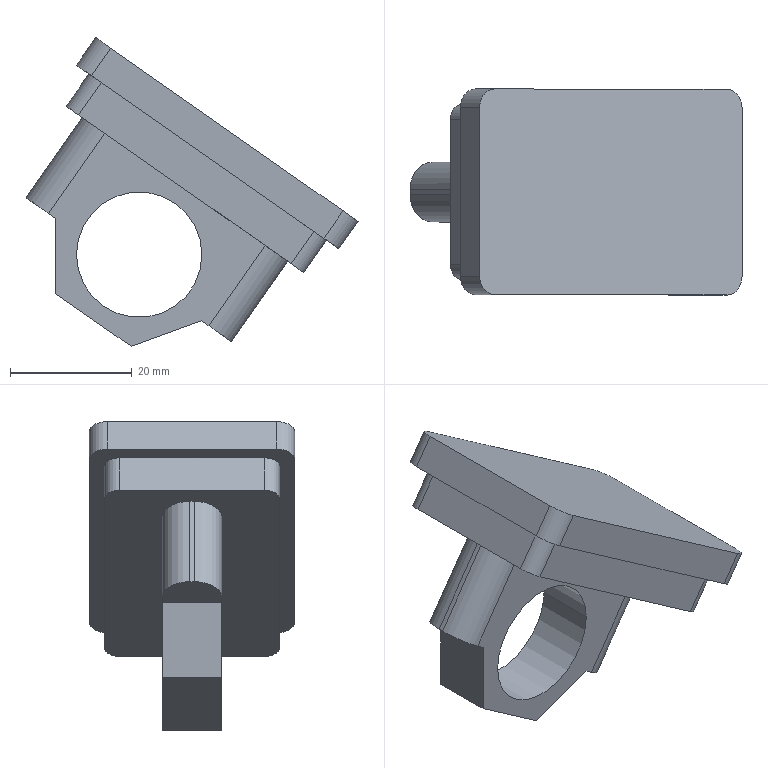Part | SolidWorks | features BaseBody 1 | 1 solid | 34 faces | box 54.536 x 33.8 x 50.697 mm | volume 23757 mm3 | plane 20 | cylinder 14 | commonest cylinder face diameters 5 x4 6 x4 9 x4 20.6 x2
STEP:
#1=CARTESIAN_POINT('',(-249.071,127.55,1106.454));
#2=VERTEX_POINT('',#1);
#3=CARTESIAN_POINT('',(-228.471,127.55,1106.454));
#4=VERTEX_POINT('',#3);
#5=CARTESIAN_POINT('',(-238.771,127.55,1106.454));
#6=DIRECTION('',(0.,-1.,0.));
#7=DIRECTION('',(-1.,0.,0.));
#8=AXIS2_PLACEMENT_3D('',#5,#6,#7);
#9=CIRCLE('',#8,10.3);
#10=EDGE_CURVE('',#2,#4,#9,.T.);
#11=ORIENTED_EDGE('',*,*,#10,.F.);
#12=CARTESIAN_POINT('',(-249.071,117.75,1106.454));
#13=VERTEX_POINT('',#12);
#14=CARTESIAN_POINT('',(-249.071,150.6,1106.454));
#15=DIRECTION('',(0.,-1.,0.));
#16=VECTOR('',#15,1000.);
#17=LINE('',#14,#16);
#18=EDGE_CURVE('',#2,#13,#17,.T.);
#19=ORIENTED_EDGE('',*,*,#18,.T.);
#20=CARTESIAN_POINT('',(-228.471,117.75,1106.454));
#21=VERTEX_POINT('',#20);
#22=CARTESIAN_POINT('',(-238.771,117.75,1106.454));
#23=DIRECTION('',(0.,-1.,0.));
#24=DIRECTION('',(1.,0.,0.));
#25=AXIS2_PLACEMENT_3D('',#22,#23,#24);
#26=CIRCLE('',#25,10.3);
#27=EDGE_CURVE('',#13,#21,#26,.T.);
#28=ORIENTED_EDGE('',*,*,#27,.T.);
#29=CARTESIAN_POINT('',(-228.471,150.6,1106.454));
#30=DIRECTION('',(0.,-1.,0.));
#31=VECTOR('',#30,1000.);
#32=LINE('',#29,#31);
#33=EDGE_CURVE('',#4,#21,#32,.T.);
#34=ORIENTED_EDGE('',*,*,#33,.F.);
#35=EDGE_LOOP('',(#11,#19,#28,#34));
#36=FACE_OUTER_BOUND('',#35,.T.);
#37=CARTESIAN_POINT('',(-238.771,150.6,1106.454));
#38=DIRECTION('',(0.,-1.,0.));
#39=DIRECTION('',(1.,0.,0.));
#40=AXIS2_PLACEMENT_3D('',#37,#38,#39);
#41=CYLINDRICAL_SURFACE('',#40,10.3);
#42=ADVANCED_FACE('',(#36),#41,.F.);
#43=CARTESIAN_POINT('',(-250.753,134.55,1130.836));
#44=VERTEX_POINT('',#43);
#45=CARTESIAN_POINT('',(-248.705,137.05,1129.402));
#46=VERTEX_POINT('',#45);
#47=CARTESIAN_POINT('',(-248.705,134.55,1129.402));
#48=DIRECTION('',(-0.5736,0.,-0.8192));
#49=DIRECTION('',(-0.8192,0.,0.5736));
#50=AXIS2_PLACEMENT_3D('',#47,#48,#49);
#51=CIRCLE('',#50,2.5);
#52=EDGE_CURVE('',#44,#46,#51,.T.);
#53=ORIENTED_EDGE('',*,*,#52,.F.);
#54=CARTESIAN_POINT('',(-247.025,134.55,1136.161));
#55=VERTEX_POINT('',#54);
#56=CARTESIAN_POINT('',(-250.753,134.55,1130.836));
#57=DIRECTION('',(-0.5736,0.,-0.8192));
#58=VECTOR('',#57,1000.);
#59=LINE('',#56,#58);
#60=EDGE_CURVE('',#55,#44,#59,.T.);
#61=ORIENTED_EDGE('',*,*,#60,.F.);
#62=CARTESIAN_POINT('',(-244.977,137.05,1134.727));
#63=VERTEX_POINT('',#62);
#64=CARTESIAN_POINT('',(-244.977,134.55,1134.727));
#65=DIRECTION('',(0.5736,0.,0.8192));
#66=DIRECTION('',(-0.8192,0.,0.5736));
#67=AXIS2_PLACEMENT_3D('',#64,#65,#66);
#68=CIRCLE('',#67,2.5);
#69=EDGE_CURVE('',#63,#55,#68,.T.);
#70=ORIENTED_EDGE('',*,*,#69,.F.);
#71=CARTESIAN_POINT('',(-248.705,137.05,1129.402));
#72=DIRECTION('',(0.5736,0.,0.8192));
#73=VECTOR('',#72,1000.);
#74=LINE('',#71,#73);
#75=EDGE_CURVE('',#46,#63,#74,.T.);
#76=ORIENTED_EDGE('',*,*,#75,.F.);
#77=EDGE_LOOP('',(#53,#61,#70,#76));
#78=FACE_OUTER_BOUND('',#77,.T.);
#79=CARTESIAN_POINT('',(-248.705,134.55,1129.402));
#80=DIRECTION('',(0.5736,0.,0.8192));
#81=DIRECTION('',(-0.8192,0.,0.5736));
#82=AXIS2_PLACEMENT_3D('',#79,#80,#81);
#83=CYLINDRICAL_SURFACE('',#82,2.5);
#84=ADVANCED_FACE('',(#78),#83,.T.);
#85=CARTESIAN_POINT('',(-248.705,108.25,1129.402));
#86=VERTEX_POINT('',#85);
#87=CARTESIAN_POINT('',(-250.753,110.75,1130.836));
#88=VERTEX_POINT('',#87);
#89=CARTESIAN_POINT('',(-248.705,110.75,1129.402));
#90=DIRECTION('',(-0.5736,0.,-0.8192));
#91=DIRECTION('',(-0.8192,0.,0.5736));
#92=AXIS2_PLACEMENT_3D('',#89,#90,#91);
#93=CIRCLE('',#92,2.5);
#94=EDGE_CURVE('',#86,#88,#93,.T.);
#95=ORIENTED_EDGE('',*,*,#94,.F.);
#96=CARTESIAN_POINT('',(-244.977,108.25,1134.727));
#97=VERTEX_POINT('',#96);
#98=CARTESIAN_POINT('',(-248.705,108.25,1129.402));
#99=DIRECTION('',(-0.5736,0.,-0.8192));
#100=VECTOR('',#99,1000.);
#101=LINE('',#98,#100);
#102=EDGE_CURVE('',#97,#86,#101,.T.);
#103=ORIENTED_EDGE('',*,*,#102,.F.);
#104=CARTESIAN_POINT('',(-247.025,110.75,1136.161));
#105=VERTEX_POINT('',#104);
#106=CARTESIAN_POINT('',(-244.977,110.75,1134.727));
#107=DIRECTION('',(0.5736,0.,0.8192));
#108=DIRECTION('',(-0.8192,0.,0.5736));
#109=AXIS2_PLACEMENT_3D('',#106,#107,#108);
#110=CIRCLE('',#109,2.5);
#111=EDGE_CURVE('',#105,#97,#110,.T.);
#112=ORIENTED_EDGE('',*,*,#111,.F.);
#113=CARTESIAN_POINT('',(-250.753,110.75,1130.836));
#114=DIRECTION('',(0.5736,0.,0.8192));
#115=VECTOR('',#114,1000.);
#116=LINE('',#113,#115);
#117=EDGE_CURVE('',#88,#105,#116,.T.);
#118=ORIENTED_EDGE('',*,*,#117,.F.);
#119=EDGE_LOOP('',(#95,#103,#112,#118));
#120=FACE_OUTER_BOUND('',#119,.T.);
#121=CARTESIAN_POINT('',(-248.705,110.75,1129.402));
#122=DIRECTION('',(0.5736,0.,0.8192));
#123=DIRECTION('',(-0.8192,0.,0.5736));
#124=AXIS2_PLACEMENT_3D('',#121,#122,#123);
#125=CYLINDRICAL_SURFACE('',#124,2.5);
#126=ADVANCED_FACE('',(#120),#125,.T.);
#127=CARTESIAN_POINT('',(-211.761,110.75,1103.534));
#128=VERTEX_POINT('',#127);
#129=CARTESIAN_POINT('',(-213.809,108.25,1104.968));
#130=VERTEX_POINT('',#129);
#131=CARTESIAN_POINT('',(-213.809,110.75,1104.968));
#132=DIRECTION('',(-0.5736,0.,-0.8192));
#133=DIRECTION('',(-0.8192,0.,0.5736));
#134=AXIS2_PLACEMENT_3D('',#131,#132,#133);
#135=CIRCLE('',#134,2.5);
#136=EDGE_CURVE('',#128,#130,#135,.T.);
#137=ORIENTED_EDGE('',*,*,#136,.F.);
#138=CARTESIAN_POINT('',(-208.033,110.75,1108.858));
#139=VERTEX_POINT('',#138);
#140=CARTESIAN_POINT('',(-211.761,110.75,1103.534));
#141=DIRECTION('',(-0.5736,0.,-0.8192));
#142=VECTOR('',#141,1000.);
#143=LINE('',#140,#142);
#144=EDGE_CURVE('',#139,#128,#143,.T.);
#145=ORIENTED_EDGE('',*,*,#144,.F.);
#146=CARTESIAN_POINT('',(-210.081,108.25,1110.292));
#147=VERTEX_POINT('',#146);
#148=CARTESIAN_POINT('',(-210.081,110.75,1110.292));
#149=DIRECTION('',(0.5736,0.,0.8192));
#150=DIRECTION('',(-0.8192,0.,0.5736));
#151=AXIS2_PLACEMENT_3D('',#148,#149,#150);
#152=CIRCLE('',#151,2.5);
#153=EDGE_CURVE('',#147,#139,#152,.T.);
#154=ORIENTED_EDGE('',*,*,#153,.F.);
#155=CARTESIAN_POINT('',(-213.809,108.25,1104.968));
#156=DIRECTION('',(0.5736,0.,0.8192));
#157=VECTOR('',#156,1000.);
#158=LINE('',#155,#157);
#159=EDGE_CURVE('',#130,#147,#158,.T.);
#160=ORIENTED_EDGE('',*,*,#159,.F.);
#161=EDGE_LOOP('',(#137,#145,#154,#160));
#162=FACE_OUTER_BOUND('',#161,.T.);
#163=CARTESIAN_POINT('',(-213.809,110.75,1104.968));
#164=DIRECTION('',(0.5736,0.,0.8192));
#165=DIRECTION('',(-0.8192,0.,0.5736));
#166=AXIS2_PLACEMENT_3D('',#163,#164,#165);
#167=CYLINDRICAL_SURFACE('',#166,2.5);
#168=ADVANCED_FACE('',(#162),#167,.T.);
#169=CARTESIAN_POINT('',(-213.809,137.05,1104.968));
#170=VERTEX_POINT('',#169);
#171=CARTESIAN_POINT('',(-211.761,134.55,1103.534));
#172=VERTEX_POINT('',#171);
#173=CARTESIAN_POINT('',(-213.809,134.55,1104.968));
#174=DIRECTION('',(-0.5736,0.,-0.8192));
#175=DIRECTION('',(-0.8192,0.,0.5736));
#176=AXIS2_PLACEMENT_3D('',#173,#174,#175);
#177=CIRCLE('',#176,2.5);
#178=EDGE_CURVE('',#170,#172,#177,.T.);
#179=ORIENTED_EDGE('',*,*,#178,.F.);
#180=CARTESIAN_POINT('',(-210.081,137.05,1110.292));
#181=VERTEX_POINT('',#180);
#182=CARTESIAN_POINT('',(-213.809,137.05,1104.968));
#183=DIRECTION('',(-0.5736,0.,-0.8192));
#184=VECTOR('',#183,1000.);
#185=LINE('',#182,#184);
#186=EDGE_CURVE('',#181,#170,#185,.T.);
#187=ORIENTED_EDGE('',*,*,#186,.F.);
#188=CARTESIAN_POINT('',(-208.033,134.55,1108.858));
#189=VERTEX_POINT('',#188);
#190=CARTESIAN_POINT('',(-210.081,134.55,1110.292));
#191=DIRECTION('',(0.5736,0.,0.8192));
#192=DIRECTION('',(-0.8192,0.,0.5736));
#193=AXIS2_PLACEMENT_3D('',#190,#191,#192);
#194=CIRCLE('',#193,2.5);
#195=EDGE_CURVE('',#189,#181,#194,.T.);
#196=ORIENTED_EDGE('',*,*,#195,.F.);
#197=CARTESIAN_POINT('',(-211.761,134.55,1103.534));
#198=DIRECTION('',(0.5736,0.,0.8192));
#199=VECTOR('',#198,1000.);
#200=LINE('',#197,#199);
#201=EDGE_CURVE('',#172,#189,#200,.T.);
#202=ORIENTED_EDGE('',*,*,#201,.F.);
#203=EDGE_LOOP('',(#179,#187,#196,#202));
#204=FACE_OUTER_BOUND('',#203,.T.);
#205=CARTESIAN_POINT('',(-213.809,134.55,1104.968));
#206=DIRECTION('',(0.5736,0.,0.8192));
#207=DIRECTION('',(-0.8192,0.,0.5736));
#208=AXIS2_PLACEMENT_3D('',#205,#206,#207);
#209=CYLINDRICAL_SURFACE('',#208,2.5);
#210=ADVANCED_FACE('',(#204),#209,.T.);
#211=CARTESIAN_POINT('',(-249.073,136.55,1137.595));
#212=VERTEX_POINT('',#211);
#213=CARTESIAN_POINT('',(-246.615,139.55,1135.874));
#214=VERTEX_POINT('',#213);
#215=CARTESIAN_POINT('',(-246.615,136.55,1135.874));
#216=DIRECTION('',(-0.5736,0.,-0.8192));
#217=DIRECTION('',(-0.8192,0.,0.5736));
#218=AXIS2_PLACEMENT_3D('',#215,#216,#217);
#219=CIRCLE('',#218,3.);
#220=EDGE_CURVE('',#212,#214,#219,.T.);
#221=ORIENTED_EDGE('',*,*,#220,.F.);
#222=CARTESIAN_POINT('',(-245.918,136.55,1142.1));
#223=VERTEX_POINT('',#222);
#224=CARTESIAN_POINT('',(-249.073,136.55,1137.595));
#225=DIRECTION('',(-0.5736,0.,-0.8192));
#226=VECTOR('',#225,1000.);
#227=LINE('',#224,#226);
#228=EDGE_CURVE('',#223,#212,#227,.T.);
#229=ORIENTED_EDGE('',*,*,#228,.F.);
#230=CARTESIAN_POINT('',(-243.461,139.55,1140.379));
#231=VERTEX_POINT('',#230);
#232=CARTESIAN_POINT('',(-243.461,136.55,1140.379));
#233=DIRECTION('',(0.5736,0.,0.8192));
#234=DIRECTION('',(-0.8192,0.,0.5736));
#235=AXIS2_PLACEMENT_3D('',#232,#233,#234);
#236=CIRCLE('',#235,3.);
#237=EDGE_CURVE('',#231,#223,#236,.T.);
#238=ORIENTED_EDGE('',*,*,#237,.F.);
#239=CARTESIAN_POINT('',(-246.615,139.55,1135.874));
#240=DIRECTION('',(0.5736,0.,0.8192));
#241=VECTOR('',#240,1000.);
#242=LINE('',#239,#241);
#243=EDGE_CURVE('',#214,#231,#242,.T.);
#244=ORIENTED_EDGE('',*,*,#243,.F.);
#245=EDGE_LOOP('',(#221,#229,#238,#244));
#246=FACE_OUTER_BOUND('',#245,.T.);
#247=CARTESIAN_POINT('',(-246.615,136.55,1135.874));
#248=DIRECTION('',(0.5736,0.,0.8192));
#249=DIRECTION('',(-0.8192,0.,0.5736));
#250=AXIS2_PLACEMENT_3D('',#247,#248,#249);
#251=CYLINDRICAL_SURFACE('',#250,3.);
#252=ADVANCED_FACE('',(#246),#251,.T.);
#253=CARTESIAN_POINT('',(-208.443,139.55,1109.145));
#254=VERTEX_POINT('',#253);
#255=CARTESIAN_POINT('',(-205.985,136.55,1107.425));
#256=VERTEX_POINT('',#255);
#257=CARTESIAN_POINT('',(-208.443,136.55,1109.145));
#258=DIRECTION('',(-0.5736,0.,-0.8192));
#259=DIRECTION('',(-0.8192,0.,0.5736));
#260=AXIS2_PLACEMENT_3D('',#257,#258,#259);
#261=CIRCLE('',#260,3.);
#262=EDGE_CURVE('',#254,#256,#261,.T.);
#263=ORIENTED_EDGE('',*,*,#262,.F.);
#264=CARTESIAN_POINT('',(-205.288,139.55,1113.651));
#265=VERTEX_POINT('',#264);
#266=CARTESIAN_POINT('',(-208.443,139.55,1109.145));
#267=DIRECTION('',(-0.5736,0.,-0.8192));
#268=VECTOR('',#267,1000.);
#269=LINE('',#266,#268);
#270=EDGE_CURVE('',#265,#254,#269,.T.);
#271=ORIENTED_EDGE('',*,*,#270,.F.);
#272=CARTESIAN_POINT('',(-202.831,136.55,1111.93));
#273=VERTEX_POINT('',#272);
#274=CARTESIAN_POINT('',(-205.288,136.55,1113.651));
#275=DIRECTION('',(0.5736,0.,0.8192));
#276=DIRECTION('',(-0.8192,0.,0.5736));
#277=AXIS2_PLACEMENT_3D('',#274,#275,#276);
#278=CIRCLE('',#277,3.);
#279=EDGE_CURVE('',#273,#265,#278,.T.);
#280=ORIENTED_EDGE('',*,*,#279,.F.);
#281=CARTESIAN_POINT('',(-205.985,136.55,1107.425));
#282=DIRECTION('',(0.5736,0.,0.8192));
#283=VECTOR('',#282,1000.);
#284=LINE('',#281,#283);
#285=EDGE_CURVE('',#256,#273,#284,.T.);
#286=ORIENTED_EDGE('',*,*,#285,.F.);
#287=EDGE_LOOP('',(#263,#271,#280,#286));
#288=FACE_OUTER_BOUND('',#287,.T.);
#289=CARTESIAN_POINT('',(-208.443,136.55,1109.145));
#290=DIRECTION('',(0.5736,0.,0.8192));
#291=DIRECTION('',(-0.8192,0.,0.5736));
#292=AXIS2_PLACEMENT_3D('',#289,#290,#291);
#293=CYLINDRICAL_SURFACE('',#292,3.);
#294=ADVANCED_FACE('',(#288),#293,.T.);
#295=CARTESIAN_POINT('',(-205.985,108.75,1107.425));
#296=VERTEX_POINT('',#295);
#297=CARTESIAN_POINT('',(-208.443,105.75,1109.145));
#298=VERTEX_POINT('',#297);
#299=CARTESIAN_POINT('',(-208.443,108.75,1109.145));
#300=DIRECTION('',(-0.5736,0.,-0.8192));
#301=DIRECTION('',(-0.8192,0.,0.5736));
#302=AXIS2_PLACEMENT_3D('',#299,#300,#301);
#303=CIRCLE('',#302,3.);
#304=EDGE_CURVE('',#296,#298,#303,.T.);
#305=ORIENTED_EDGE('',*,*,#304,.F.);
#306=CARTESIAN_POINT('',(-202.831,108.75,1111.93));
#307=VERTEX_POINT('',#306);
#308=CARTESIAN_POINT('',(-205.985,108.75,1107.425));
#309=DIRECTION('',(-0.5736,0.,-0.8192));
#310=VECTOR('',#309,1000.);
#311=LINE('',#308,#310);
#312=EDGE_CURVE('',#307,#296,#311,.T.);
#313=ORIENTED_EDGE('',*,*,#312,.F.);
#314=CARTESIAN_POINT('',(-205.288,105.75,1113.651));
#315=VERTEX_POINT('',#314);
#316=CARTESIAN_POINT('',(-205.288,108.75,1113.651));
#317=DIRECTION('',(0.5736,0.,0.8192));
#318=DIRECTION('',(-0.8192,0.,0.5736));
#319=AXIS2_PLACEMENT_3D('',#316,#317,#318);
#320=CIRCLE('',#319,3.);
#321=EDGE_CURVE('',#315,#307,#320,.T.);
#322=ORIENTED_EDGE('',*,*,#321,.F.);
#323=CARTESIAN_POINT('',(-208.443,105.75,1109.145));
#324=DIRECTION('',(0.5736,0.,0.8192));
#325=VECTOR('',#324,1000.);
#326=LINE('',#323,#325);
#327=EDGE_CURVE('',#298,#315,#326,.T.);
#328=ORIENTED_EDGE('',*,*,#327,.F.);
#329=EDGE_LOOP('',(#305,#313,#322,#328));
#330=FACE_OUTER_BOUND('',#329,.T.);
#331=CARTESIAN_POINT('',(-208.443,108.75,1109.145));
#332=DIRECTION('',(0.5736,0.,0.8192));
#333=DIRECTION('',(-0.8192,0.,0.5736));
#334=AXIS2_PLACEMENT_3D('',#331,#332,#333);
#335=CYLINDRICAL_SURFACE('',#334,3.);
#336=ADVANCED_FACE('',(#330),#335,.T.);
#337=CARTESIAN_POINT('',(-246.615,105.75,1135.874));
#338=VERTEX_POINT('',#337);
#339=CARTESIAN_POINT('',(-249.073,108.75,1137.595));
#340=VERTEX_POINT('',#339);
#341=CARTESIAN_POINT('',(-246.615,108.75,1135.874));
#342=DIRECTION('',(-0.5736,0.,-0.8192));
#343=DIRECTION('',(-0.8192,0.,0.5736));
#344=AXIS2_PLACEMENT_3D('',#341,#342,#343);
#345=CIRCLE('',#344,3.);
#346=EDGE_CURVE('',#338,#340,#345,.T.);
#347=ORIENTED_EDGE('',*,*,#346,.F.);
#348=CARTESIAN_POINT('',(-243.461,105.75,1140.379));
#349=VERTEX_POINT('',#348);
#350=CARTESIAN_POINT('',(-246.615,105.75,1135.874));
#351=DIRECTION('',(-0.5736,0.,-0.8192));
#352=VECTOR('',#351,1000.);
#353=LINE('',#350,#352);
#354=EDGE_CURVE('',#349,#338,#353,.T.);
#355=ORIENTED_EDGE('',*,*,#354,.F.);
#356=CARTESIAN_POINT('',(-245.918,108.75,1142.1));
#357=VERTEX_POINT('',#356);
#358=CARTESIAN_POINT('',(-243.461,108.75,1140.379));
#359=DIRECTION('',(0.5736,0.,0.8192));
#360=DIRECTION('',(-0.8192,0.,0.5736));
#361=AXIS2_PLACEMENT_3D('',#358,#359,#360);
#362=CIRCLE('',#361,3.);
#363=EDGE_CURVE('',#357,#349,#362,.T.);
#364=ORIENTED_EDGE('',*,*,#363,.F.);
#365=CARTESIAN_POINT('',(-249.073,108.75,1137.595));
#366=DIRECTION('',(0.5736,0.,0.8192));
#367=VECTOR('',#366,1000.);
#368=LINE('',#365,#367);
#369=EDGE_CURVE('',#340,#357,#368,.T.);
#370=ORIENTED_EDGE('',*,*,#369,.F.);
#371=EDGE_LOOP('',(#347,#355,#364,#370));
#372=FACE_OUTER_BOUND('',#371,.T.);
#373=CARTESIAN_POINT('',(-246.615,108.75,1135.874));
#374=DIRECTION('',(0.5736,0.,0.8192));
#375=DIRECTION('',(-0.8192,0.,0.5736));
#376=AXIS2_PLACEMENT_3D('',#373,#374,#375);
#377=CYLINDRICAL_SURFACE('',#376,3.);
#378=ADVANCED_FACE('',(#372),#377,.T.);
#379=CARTESIAN_POINT('',(-252.455,127.55,1112.373));
#380=VERTEX_POINT('',#379);
#381=CARTESIAN_POINT('',(-252.455,117.75,1112.373));
#382=VERTEX_POINT('',#381);
#383=CARTESIAN_POINT('',(-252.455,235.55,1112.373));
#384=DIRECTION('',(0.,-1.,0.));
#385=VECTOR('',#384,1000.);
#386=LINE('',#383,#385);
#387=EDGE_CURVE('',#380,#382,#386,.T.);
#388=ORIENTED_EDGE('',*,*,#387,.T.);
#389=CARTESIAN_POINT('',(-253.68,117.75,1113.231));
#390=VERTEX_POINT('',#389);
#391=CARTESIAN_POINT('',(-240.492,117.75,1103.997));
#392=DIRECTION('',(0.8192,0.,-0.5736));
#393=VECTOR('',#392,1000.);
#394=LINE('',#391,#393);
#395=EDGE_CURVE('',#390,#382,#394,.T.);
#396=ORIENTED_EDGE('',*,*,#395,.F.);
#397=CARTESIAN_POINT('',(-257.366,122.25,1115.812));
#398=VERTEX_POINT('',#397);
#399=CARTESIAN_POINT('',(-253.68,122.25,1113.231));
#400=DIRECTION('',(0.5736,0.,0.8192));
#401=DIRECTION('',(-0.8192,0.,0.5736));
#402=AXIS2_PLACEMENT_3D('',#399,#400,#401);
#403=CIRCLE('',#402,4.5);
#404=EDGE_CURVE('',#398,#390,#403,.T.);
#405=ORIENTED_EDGE('',*,*,#404,.F.);
#406=CARTESIAN_POINT('',(-257.366,123.05,1115.812));
#407=VERTEX_POINT('',#406);
#408=CARTESIAN_POINT('',(-257.366,134.05,1115.812));
#409=DIRECTION('',(0.,1.,0.));
#410=VECTOR('',#409,1000.);
#411=LINE('',#408,#410);
#412=EDGE_CURVE('',#398,#407,#411,.T.);
#413=ORIENTED_EDGE('',*,*,#412,.T.);
#414=CARTESIAN_POINT('',(-253.68,127.55,1113.231));
#415=VERTEX_POINT('',#414);
#416=CARTESIAN_POINT('',(-253.68,123.05,1113.231));
#417=DIRECTION('',(0.5736,0.,0.8192));
#418=DIRECTION('',(-0.8192,0.,0.5736));
#419=AXIS2_PLACEMENT_3D('',#416,#417,#418);
#420=CIRCLE('',#419,4.5);
#421=EDGE_CURVE('',#415,#407,#420,.T.);
#422=ORIENTED_EDGE('',*,*,#421,.F.);
#423=CARTESIAN_POINT('',(439.589,127.55,627.799));
#424=DIRECTION('',(0.8192,0.,-0.5736));
#425=VECTOR('',#424,1000.);
#426=LINE('',#423,#425);
#427=EDGE_CURVE('',#415,#380,#426,.T.);
#428=ORIENTED_EDGE('',*,*,#427,.T.);
#429=EDGE_LOOP('',(#388,#396,#405,#413,#422,#428));
#430=FACE_OUTER_BOUND('',#429,.T.);
#431=CARTESIAN_POINT('',(-252.455,235.55,1112.373));
#432=DIRECTION('',(-0.5736,0.,-0.8192));
#433=DIRECTION('',(-0.8192,0.,0.5736));
#434=AXIS2_PLACEMENT_3D('',#431,#432,#433);
#435=PLANE('',#434);
#436=ADVANCED_FACE('',(#430),#435,.T.);
#437=CARTESIAN_POINT('',(-252.455,127.55,1100.043));
#438=VERTEX_POINT('',#437);
#439=CARTESIAN_POINT('',(-252.455,117.75,1100.043));
#440=VERTEX_POINT('',#439);
#441=CARTESIAN_POINT('',(-252.455,122.65,1100.043));
#442=DIRECTION('',(0.,-1.,0.));
#443=VECTOR('',#442,1000.);
#444=LINE('',#441,#443);
#445=EDGE_CURVE('',#438,#440,#444,.T.);
#446=ORIENTED_EDGE('',*,*,#445,.T.);
#447=CARTESIAN_POINT('',(-252.455,117.75,1122.51));
#448=DIRECTION('',(0.,0.,-1.));
#449=VECTOR('',#448,1000.);
#450=LINE('',#447,#449);
#451=EDGE_CURVE('',#382,#440,#450,.T.);
#452=ORIENTED_EDGE('',*,*,#451,.F.);
#453=ORIENTED_EDGE('',*,*,#387,.F.);
#454=CARTESIAN_POINT('',(-252.455,127.55,-21.38));
#455=DIRECTION('',(0.,0.,-1.));
#456=VECTOR('',#455,1000.);
#457=LINE('',#454,#456);
#458=EDGE_CURVE('',#380,#438,#457,.T.);
#459=ORIENTED_EDGE('',*,*,#458,.T.);
#460=EDGE_LOOP('',(#446,#452,#453,#459));
#461=FACE_OUTER_BOUND('',#460,.T.);
#462=CARTESIAN_POINT('',(-252.455,235.55,1112.373));
#463=DIRECTION('',(-1.,0.,0.));
#464=DIRECTION('',(0.,0.,1.));
#465=AXIS2_PLACEMENT_3D('',#462,#463,#464);
#466=PLANE('',#465);
#467=ADVANCED_FACE('',(#461),#466,.T.);
#468=CARTESIAN_POINT('',(-227.303,117.75,1094.762));
#469=VERTEX_POINT('',#468);
#470=CARTESIAN_POINT('',(-223.617,122.25,1092.181));
#471=VERTEX_POINT('',#470);
#472=CARTESIAN_POINT('',(-227.303,122.25,1094.762));
#473=DIRECTION('',(0.5736,0.,0.8192));
#474=DIRECTION('',(-0.8192,0.,0.5736));
#475=AXIS2_PLACEMENT_3D('',#472,#473,#474);
#476=CIRCLE('',#475,4.5);
#477=EDGE_CURVE('',#469,#471,#476,.T.);
#478=ORIENTED_EDGE('',*,*,#477,.F.);
#479=CARTESIAN_POINT('',(-228.529,117.75,1095.62));
#480=VERTEX_POINT('',#479);
#481=CARTESIAN_POINT('',(-240.492,117.75,1103.997));
#482=DIRECTION('',(0.8192,0.,-0.5736));
#483=VECTOR('',#482,1000.);
#484=LINE('',#481,#483);
#485=EDGE_CURVE('',#480,#469,#484,.T.);
#486=ORIENTED_EDGE('',*,*,#485,.F.);
#487=CARTESIAN_POINT('',(-228.529,127.55,1095.62));
#488=VERTEX_POINT('',#487);
#489=CARTESIAN_POINT('',(-228.529,235.55,1095.62));
#490=DIRECTION('',(0.,-1.,0.));
#491=VECTOR('',#490,1000.);
#492=LINE('',#489,#491);
#493=EDGE_CURVE('',#488,#480,#492,.T.);
#494=ORIENTED_EDGE('',*,*,#493,.F.);
#495=CARTESIAN_POINT('',(-227.303,127.55,1094.762));
#496=VERTEX_POINT('',#495);
#497=CARTESIAN_POINT('',(439.589,127.55,627.799));
#498=DIRECTION('',(0.8192,0.,-0.5736));
#499=VECTOR('',#498,1000.);
#500=LINE('',#497,#499);
#501=EDGE_CURVE('',#488,#496,#500,.T.);
#502=ORIENTED_EDGE('',*,*,#501,.T.);
#503=CARTESIAN_POINT('',(-223.617,123.05,1092.181));
#504=VERTEX_POINT('',#503);
#505=CARTESIAN_POINT('',(-227.303,123.05,1094.762));
#506=DIRECTION('',(0.5736,0.,0.8192));
#507=DIRECTION('',(-0.8192,0.,0.5736));
#508=AXIS2_PLACEMENT_3D('',#505,#506,#507);
#509=CIRCLE('',#508,4.5);
#510=EDGE_CURVE('',#504,#496,#509,.T.);
#511=ORIENTED_EDGE('',*,*,#510,.F.);
#512=CARTESIAN_POINT('',(-223.617,134.05,1092.181));
#513=DIRECTION('',(0.,-1.,0.));
#514=VECTOR('',#513,1000.);
#515=LINE('',#512,#514);
#516=EDGE_CURVE('',#504,#471,#515,.T.);
#517=ORIENTED_EDGE('',*,*,#516,.T.);
#518=EDGE_LOOP('',(#478,#486,#494,#502,#511,#517));
#519=FACE_OUTER_BOUND('',#518,.T.);
#520=CARTESIAN_POINT('',(-216.531,235.55,1087.219));
#521=DIRECTION('',(-0.5736,0.,-0.8192));
#522=DIRECTION('',(-0.8192,0.,0.5736));
#523=AXIS2_PLACEMENT_3D('',#520,#521,#522);
#524=PLANE('',#523);
#525=ADVANCED_FACE('',(#519),#524,.T.);
#526=ORIENTED_EDGE('',*,*,#493,.T.);
#527=CARTESIAN_POINT('',(-240.115,117.75,1091.403));
#528=VERTEX_POINT('',#527);
#529=CARTESIAN_POINT('',(-219.004,117.75,1099.087));
#530=DIRECTION('',(0.9397,0.,0.342));
#531=VECTOR('',#530,1000.);
#532=LINE('',#529,#531);
#533=EDGE_CURVE('',#528,#480,#532,.T.);
#534=ORIENTED_EDGE('',*,*,#533,.F.);
#535=CARTESIAN_POINT('',(-240.115,127.55,1091.403));
#536=VERTEX_POINT('',#535);
#537=CARTESIAN_POINT('',(-240.115,122.65,1091.403));
#538=DIRECTION('',(0.,1.,0.));
#539=VECTOR('',#538,1000.);
#540=LINE('',#537,#539);
#541=EDGE_CURVE('',#528,#536,#540,.T.);
#542=ORIENTED_EDGE('',*,*,#541,.T.);
#543=CARTESIAN_POINT('',(-398.949,127.55,1033.593));
#544=DIRECTION('',(0.9397,0.,0.342));
#545=VECTOR('',#544,1000.);
#546=LINE('',#543,#545);
#547=EDGE_CURVE('',#536,#488,#546,.T.);
#548=ORIENTED_EDGE('',*,*,#547,.T.);
#549=EDGE_LOOP('',(#526,#534,#542,#548));
#550=FACE_OUTER_BOUND('',#549,.T.);
#551=CARTESIAN_POINT('',(-228.529,235.55,1095.62));
#552=DIRECTION('',(0.342,0.,-0.9397));
#553=DIRECTION('',(0.,-1.,0.));
#554=AXIS2_PLACEMENT_3D('',#551,#552,#553);
#555=PLANE('',#554);
#556=ADVANCED_FACE('',(#550),#555,.T.);
#557=ORIENTED_EDGE('',*,*,#445,.F.);
#558=CARTESIAN_POINT('',(433.796,127.55,619.525));
#559=DIRECTION('',(0.8192,0.,-0.5736));
#560=VECTOR('',#559,1000.);
#561=LINE('',#558,#560);
#562=EDGE_CURVE('',#438,#536,#561,.T.);
#563=ORIENTED_EDGE('',*,*,#562,.T.);
#564=ORIENTED_EDGE('',*,*,#541,.F.);
#565=CARTESIAN_POINT('',(-246.285,117.75,1095.723));
#566=DIRECTION('',(0.8192,0.,-0.5736));
#567=VECTOR('',#566,1000.);
#568=LINE('',#565,#567);
#569=EDGE_CURVE('',#440,#528,#568,.T.);
#570=ORIENTED_EDGE('',*,*,#569,.F.);
#571=EDGE_LOOP('',(#557,#563,#564,#570));
#572=FACE_OUTER_BOUND('',#571,.T.);
#573=CARTESIAN_POINT('',(-246.285,122.65,1095.723));
#574=DIRECTION('',(0.5736,0.,0.8192));
#575=DIRECTION('',(0.,-1.,0.));
#576=AXIS2_PLACEMENT_3D('',#573,#574,#575);
#577=PLANE('',#576);
#578=ADVANCED_FACE('',(#572),#577,.F.);
#579=CARTESIAN_POINT('',(-248.132,122.25,1129.001));
#580=VERTEX_POINT('',#579);
#581=CARTESIAN_POINT('',(-256.735,122.25,1116.714));
#582=DIRECTION('',(0.5736,0.,0.8192));
#583=VECTOR('',#582,1000.);
#584=LINE('',#581,#583);
#585=EDGE_CURVE('',#398,#580,#584,.T.);
#586=ORIENTED_EDGE('',*,*,#585,.T.);
#587=CARTESIAN_POINT('',(-248.132,123.05,1129.001));
#588=VERTEX_POINT('',#587);
#589=CARTESIAN_POINT('',(-248.132,134.05,1129.001));
#590=DIRECTION('',(0.,1.,0.));
#591=VECTOR('',#590,1000.);
#592=LINE('',#589,#591);
#593=EDGE_CURVE('',#580,#588,#592,.T.);
#594=ORIENTED_EDGE('',*,*,#593,.T.);
#595=CARTESIAN_POINT('',(-248.419,123.05,1128.591));
#596=DIRECTION('',(-0.5736,0.,-0.8192));
#597=VECTOR('',#596,1000.);
#598=LINE('',#595,#597);
#599=EDGE_CURVE('',#588,#407,#598,.T.);
#600=ORIENTED_EDGE('',*,*,#599,.T.);
#601=ORIENTED_EDGE('',*,*,#412,.F.);
#602=EDGE_LOOP('',(#586,#594,#600,#601));
#603=FACE_OUTER_BOUND('',#602,.T.);
#604=CARTESIAN_POINT('',(-248.419,134.05,1128.591));
#605=DIRECTION('',(0.8192,0.,-0.5736));
#606=DIRECTION('',(0.,-1.,0.));
#607=AXIS2_PLACEMENT_3D('',#604,#605,#606);
#608=PLANE('',#607);
#609=ADVANCED_FACE('',(#603),#608,.F.);
#610=CARTESIAN_POINT('',(-214.383,123.05,1105.369));
#611=VERTEX_POINT('',#610);
#612=CARTESIAN_POINT('',(-207.5,123.05,1115.199));
#613=DIRECTION('',(0.5736,0.,0.8192));
#614=VECTOR('',#613,1000.);
#615=LINE('',#612,#614);
#616=EDGE_CURVE('',#504,#611,#615,.T.);
#617=ORIENTED_EDGE('',*,*,#616,.T.);
#618=CARTESIAN_POINT('',(-214.383,122.25,1105.369));
#619=VERTEX_POINT('',#618);
#620=CARTESIAN_POINT('',(-214.383,134.05,1105.369));
#621=DIRECTION('',(0.,-1.,0.));
#622=VECTOR('',#621,1000.);
#623=LINE('',#620,#622);
#624=EDGE_CURVE('',#611,#619,#623,.T.);
#625=ORIENTED_EDGE('',*,*,#624,.T.);
#626=CARTESIAN_POINT('',(-207.5,122.25,1115.199));
#627=DIRECTION('',(-0.5736,0.,-0.8192));
#628=VECTOR('',#627,1000.);
#629=LINE('',#626,#628);
#630=EDGE_CURVE('',#619,#471,#629,.T.);
#631=ORIENTED_EDGE('',*,*,#630,.T.);
#632=ORIENTED_EDGE('',*,*,#516,.F.);
#633=EDGE_LOOP('',(#617,#625,#631,#632));
#634=FACE_OUTER_BOUND('',#633,.T.);
#635=CARTESIAN_POINT('',(-207.5,134.05,1115.199));
#636=DIRECTION('',(-0.8192,0.,0.5736));
#637=DIRECTION('',(0.,1.,0.));
#638=AXIS2_PLACEMENT_3D('',#635,#636,#637);
#639=PLANE('',#638);
#640=ADVANCED_FACE('',(#634),#639,.F.);
#641=CARTESIAN_POINT('',(-238.771,127.55,1106.454));
#642=DIRECTION('',(0.,-1.,0.));
#643=DIRECTION('',(-1.,0.,0.));
#644=AXIS2_PLACEMENT_3D('',#641,#642,#643);
#645=CIRCLE('',#644,10.3);
#646=EDGE_CURVE('',#4,#2,#645,.T.);
#647=ORIENTED_EDGE('',*,*,#646,.T.);
#648=ORIENTED_EDGE('',*,*,#10,.T.);
#649=EDGE_LOOP('',(#647,#648));
#650=FACE_BOUND('',#649,.T.);
#651=ORIENTED_EDGE('',*,*,#501,.F.);
#652=ORIENTED_EDGE('',*,*,#547,.F.);
#653=ORIENTED_EDGE('',*,*,#562,.F.);
#654=ORIENTED_EDGE('',*,*,#458,.F.);
#655=ORIENTED_EDGE('',*,*,#427,.F.);
#656=CARTESIAN_POINT('',(-244.446,127.55,1126.42));
#657=VERTEX_POINT('',#656);
#658=CARTESIAN_POINT('',(-708.24,127.55,464.053));
#659=DIRECTION('',(0.5736,0.,0.8192));
#660=VECTOR('',#659,1000.);
#661=LINE('',#658,#660);
#662=EDGE_CURVE('',#415,#657,#661,.T.);
#663=ORIENTED_EDGE('',*,*,#662,.T.);
#664=CARTESIAN_POINT('',(-218.069,127.55,1107.951));
#665=VERTEX_POINT('',#664);
#666=CARTESIAN_POINT('',(448.824,127.55,640.987));
#667=DIRECTION('',(0.8192,0.,-0.5736));
#668=VECTOR('',#667,1000.);
#669=LINE('',#666,#668);
#670=EDGE_CURVE('',#657,#665,#669,.T.);
#671=ORIENTED_EDGE('',*,*,#670,.T.);
#672=CARTESIAN_POINT('',(-681.863,127.55,445.584));
#673=DIRECTION('',(-0.5736,0.,-0.8192));
#674=VECTOR('',#673,1000.);
#675=LINE('',#672,#674);
#676=EDGE_CURVE('',#665,#496,#675,.T.);
#677=ORIENTED_EDGE('',*,*,#676,.T.);
#678=EDGE_LOOP('',(#651,#652,#653,#654,#655,#663,#671,#677));
#679=FACE_OUTER_BOUND('',#678,.T.);
#680=CARTESIAN_POINT('',(-14.97,127.55,-21.38));
#681=DIRECTION('',(0.,-1.,0.));
#682=DIRECTION('',(0.,0.,-1.));
#683=AXIS2_PLACEMENT_3D('',#680,#681,#682);
#684=PLANE('',#683);
#685=ADVANCED_FACE('',(#650,#679),#684,.F.);
#686=ORIENTED_EDGE('',*,*,#676,.F.);
#687=CARTESIAN_POINT('',(-218.069,123.05,1107.951));
#688=DIRECTION('',(0.5736,0.,0.8192));
#689=DIRECTION('',(-0.8192,0.,0.5736));
#690=AXIS2_PLACEMENT_3D('',#687,#688,#689);
#691=CIRCLE('',#690,4.5);
#692=EDGE_CURVE('',#611,#665,#691,.T.);
#693=ORIENTED_EDGE('',*,*,#692,.F.);
#694=ORIENTED_EDGE('',*,*,#616,.F.);
#695=ORIENTED_EDGE('',*,*,#510,.T.);
#696=EDGE_LOOP('',(#686,#693,#694,#695));
#697=FACE_OUTER_BOUND('',#696,.T.);
#698=CARTESIAN_POINT('',(-211.186,123.05,1117.78));
#699=DIRECTION('',(-0.5736,0.,-0.8192));
#700=DIRECTION('',(0.8192,0.,-0.5736));
#701=AXIS2_PLACEMENT_3D('',#698,#699,#700);
#702=CYLINDRICAL_SURFACE('',#701,4.5);
#703=ADVANCED_FACE('',(#697),#702,.T.);
#704=ORIENTED_EDGE('',*,*,#599,.F.);
#705=CARTESIAN_POINT('',(-244.446,123.05,1126.42));
#706=DIRECTION('',(0.5736,0.,0.8192));
#707=DIRECTION('',(-0.8192,0.,0.5736));
#708=AXIS2_PLACEMENT_3D('',#705,#706,#707);
#709=CIRCLE('',#708,4.5);
#710=EDGE_CURVE('',#657,#588,#709,.T.);
#711=ORIENTED_EDGE('',*,*,#710,.F.);
#712=ORIENTED_EDGE('',*,*,#662,.F.);
#713=ORIENTED_EDGE('',*,*,#421,.T.);
#714=EDGE_LOOP('',(#704,#711,#712,#713));
#715=FACE_OUTER_BOUND('',#714,.T.);
#716=CARTESIAN_POINT('',(-244.732,123.05,1126.01));
#717=DIRECTION('',(0.5736,0.,0.8192));
#718=DIRECTION('',(-0.8192,0.,0.5736));
#719=AXIS2_PLACEMENT_3D('',#716,#717,#718);
#720=CYLINDRICAL_SURFACE('',#719,4.5);
#721=ADVANCED_FACE('',(#715),#720,.T.);
#722=CARTESIAN_POINT('',(-238.771,117.75,1106.454));
#723=DIRECTION('',(0.,-1.,0.));
#724=DIRECTION('',(1.,0.,0.));
#725=AXIS2_PLACEMENT_3D('',#722,#723,#724);
#726=CIRCLE('',#725,10.3);
#727=EDGE_CURVE('',#21,#13,#726,.T.);
#728=ORIENTED_EDGE('',*,*,#727,.F.);
#729=ORIENTED_EDGE('',*,*,#27,.F.);
#730=EDGE_LOOP('',(#728,#729));
#731=FACE_BOUND('',#730,.T.);
#732=CARTESIAN_POINT('',(-218.069,117.75,1107.951));
#733=VERTEX_POINT('',#732);
#734=CARTESIAN_POINT('',(-226.672,117.75,1095.663));
#735=DIRECTION('',(0.5736,0.,0.8192));
#736=VECTOR('',#735,1000.);
#737=LINE('',#734,#736);
#738=EDGE_CURVE('',#469,#733,#737,.T.);
#739=ORIENTED_EDGE('',*,*,#738,.T.);
#740=CARTESIAN_POINT('',(-244.446,117.75,1126.42));
#741=VERTEX_POINT('',#740);
#742=CARTESIAN_POINT('',(-231.257,117.75,1117.185));
#743=DIRECTION('',(0.8192,0.,-0.5736));
#744=VECTOR('',#743,1000.);
#745=LINE('',#742,#744);
#746=EDGE_CURVE('',#741,#733,#745,.T.);
#747=ORIENTED_EDGE('',*,*,#746,.F.);
#748=CARTESIAN_POINT('',(-237.563,117.75,1136.25));
#749=DIRECTION('',(-0.5736,0.,-0.8192));
#750=VECTOR('',#749,1000.);
#751=LINE('',#748,#750);
#752=EDGE_CURVE('',#741,#390,#751,.T.);
#753=ORIENTED_EDGE('',*,*,#752,.T.);
#754=ORIENTED_EDGE('',*,*,#395,.T.);
#755=ORIENTED_EDGE('',*,*,#451,.T.);
#756=ORIENTED_EDGE('',*,*,#569,.T.);
#757=ORIENTED_EDGE('',*,*,#533,.T.);
#758=ORIENTED_EDGE('',*,*,#485,.T.);
#759=EDGE_LOOP('',(#739,#747,#753,#754,#755,#756,#757,#758));
#760=FACE_OUTER_BOUND('',#759,.T.);
#761=CARTESIAN_POINT('',(-227.529,117.75,1122.51));
#762=DIRECTION('',(0.,1.,0.));
#763=DIRECTION('',(1.,0.,0.));
#764=AXIS2_PLACEMENT_3D('',#761,#762,#763);
#765=PLANE('',#764);
#766=ADVANCED_FACE('',(#731,#760),#765,.F.);
#767=ORIENTED_EDGE('',*,*,#752,.F.);
#768=CARTESIAN_POINT('',(-244.446,122.25,1126.42));
#769=DIRECTION('',(0.5736,0.,0.8192));
#770=DIRECTION('',(-0.8192,0.,0.5736));
#771=AXIS2_PLACEMENT_3D('',#768,#769,#770);
#772=CIRCLE('',#771,4.5);
#773=EDGE_CURVE('',#580,#741,#772,.T.);
#774=ORIENTED_EDGE('',*,*,#773,.F.);
#775=ORIENTED_EDGE('',*,*,#585,.F.);
#776=ORIENTED_EDGE('',*,*,#404,.T.);
#777=EDGE_LOOP('',(#767,#774,#775,#776));
#778=FACE_OUTER_BOUND('',#777,.T.);
#779=CARTESIAN_POINT('',(-240.717,122.25,1131.744));
#780=DIRECTION('',(0.5736,0.,0.8192));
#781=DIRECTION('',(-0.8192,0.,0.5736));
#782=AXIS2_PLACEMENT_3D('',#779,#780,#781);
#783=CYLINDRICAL_SURFACE('',#782,4.5);
#784=ADVANCED_FACE('',(#778),#783,.T.);
#785=ORIENTED_EDGE('',*,*,#630,.F.);
#786=CARTESIAN_POINT('',(-218.069,122.25,1107.951));
#787=DIRECTION('',(0.5736,0.,0.8192));
#788=DIRECTION('',(-0.8192,0.,0.5736));
#789=AXIS2_PLACEMENT_3D('',#786,#787,#788);
#790=CIRCLE('',#789,4.5);
#791=EDGE_CURVE('',#733,#619,#790,.T.);
#792=ORIENTED_EDGE('',*,*,#791,.F.);
#793=ORIENTED_EDGE('',*,*,#738,.F.);
#794=ORIENTED_EDGE('',*,*,#477,.T.);
#795=EDGE_LOOP('',(#785,#792,#793,#794));
#796=FACE_OUTER_BOUND('',#795,.T.);
#797=CARTESIAN_POINT('',(-214.341,122.25,1113.275));
#798=DIRECTION('',(-0.5736,0.,-0.8192));
#799=DIRECTION('',(0.8192,0.,-0.5736));
#800=AXIS2_PLACEMENT_3D('',#797,#798,#799);
#801=CYLINDRICAL_SURFACE('',#800,4.5);
#802=ADVANCED_FACE('',(#796),#801,.T.);
#803=CARTESIAN_POINT('',(-224.374,105.75,1127.015));
#804=DIRECTION('',(-0.8192,0.,0.5736));
#805=VECTOR('',#804,1000.);
#806=LINE('',#803,#805);
#807=EDGE_CURVE('',#315,#349,#806,.T.);
#808=ORIENTED_EDGE('',*,*,#807,.F.);
#809=ORIENTED_EDGE('',*,*,#321,.T.);
#810=CARTESIAN_POINT('',(-202.831,105.75,1111.93));
#811=DIRECTION('',(0.,-1.,0.));
#812=VECTOR('',#811,1000.);
#813=LINE('',#810,#812);
#814=EDGE_CURVE('',#273,#307,#813,.T.);
#815=ORIENTED_EDGE('',*,*,#814,.F.);
#816=ORIENTED_EDGE('',*,*,#279,.T.);
#817=CARTESIAN_POINT('',(-202.831,139.55,1111.93));
#818=DIRECTION('',(0.8192,0.,-0.5736));
#819=VECTOR('',#818,1000.);
#820=LINE('',#817,#819);
#821=EDGE_CURVE('',#231,#265,#820,.T.);
#822=ORIENTED_EDGE('',*,*,#821,.F.);
#823=ORIENTED_EDGE('',*,*,#237,.T.);
#824=CARTESIAN_POINT('',(-245.918,139.55,1142.1));
#825=DIRECTION('',(0.,1.,0.));
#826=VECTOR('',#825,1000.);
#827=LINE('',#824,#826);
#828=EDGE_CURVE('',#357,#223,#827,.T.);
#829=ORIENTED_EDGE('',*,*,#828,.F.);
#830=ORIENTED_EDGE('',*,*,#363,.T.);
#831=EDGE_LOOP('',(#808,#809,#815,#816,#822,#823,#829,#830));
#832=FACE_OUTER_BOUND('',#831,.T.);
#833=CARTESIAN_POINT('',(-241.249,134.05,1138.831));
#834=DIRECTION('',(-0.5736,0.,-0.8192));
#835=DIRECTION('',(-0.8192,0.,0.5736));
#836=AXIS2_PLACEMENT_3D('',#833,#834,#835);
#837=PLANE('',#836);
#838=ADVANCED_FACE('',(#832),#837,.F.);
#839=ORIENTED_EDGE('',*,*,#670,.F.);
#840=ORIENTED_EDGE('',*,*,#710,.T.);
#841=ORIENTED_EDGE('',*,*,#593,.F.);
#842=ORIENTED_EDGE('',*,*,#773,.T.);
#843=ORIENTED_EDGE('',*,*,#746,.T.);
#844=ORIENTED_EDGE('',*,*,#791,.T.);
#845=ORIENTED_EDGE('',*,*,#624,.F.);
#846=ORIENTED_EDGE('',*,*,#692,.T.);
#847=EDGE_LOOP('',(#839,#840,#841,#842,#843,#844,#845,#846));
#848=FACE_BOUND('',#847,.T.);
#849=CARTESIAN_POINT('',(-211.761,105.75,1103.534));
#850=DIRECTION('',(0.,-1.,0.));
#851=VECTOR('',#850,1000.);
#852=LINE('',#849,#851);
#853=EDGE_CURVE('',#172,#128,#852,.T.);
#854=ORIENTED_EDGE('',*,*,#853,.T.);
#855=ORIENTED_EDGE('',*,*,#136,.T.);
#856=CARTESIAN_POINT('',(-252.801,108.25,1132.27));
#857=DIRECTION('',(-0.8192,0.,0.5736));
#858=VECTOR('',#857,1000.);
#859=LINE('',#856,#858);
#860=EDGE_CURVE('',#130,#86,#859,.T.);
#861=ORIENTED_EDGE('',*,*,#860,.T.);
#862=ORIENTED_EDGE('',*,*,#94,.T.);
#863=CARTESIAN_POINT('',(-250.753,139.55,1130.836));
#864=DIRECTION('',(0.,1.,0.));
#865=VECTOR('',#864,1000.);
#866=LINE('',#863,#865);
#867=EDGE_CURVE('',#88,#44,#866,.T.);
#868=ORIENTED_EDGE('',*,*,#867,.T.);
#869=ORIENTED_EDGE('',*,*,#52,.T.);
#870=CARTESIAN_POINT('',(-209.713,137.05,1102.1));
#871=DIRECTION('',(0.8192,0.,-0.5736));
#872=VECTOR('',#871,1000.);
#873=LINE('',#870,#872);
#874=EDGE_CURVE('',#46,#170,#873,.T.);
#875=ORIENTED_EDGE('',*,*,#874,.T.);
#876=ORIENTED_EDGE('',*,*,#178,.T.);
#877=EDGE_LOOP('',(#854,#855,#861,#862,#868,#869,#875,#876));
#878=FACE_OUTER_BOUND('',#877,.T.);
#879=CARTESIAN_POINT('',(448.824,-8.3,640.987));
#880=DIRECTION('',(-0.5736,0.,-0.8192));
#881=DIRECTION('',(-0.8192,0.,0.5736));
#882=AXIS2_PLACEMENT_3D('',#879,#880,#881);
#883=PLANE('',#882);
#884=ADVANCED_FACE('',(#848,#878),#883,.T.);
#885=CARTESIAN_POINT('',(-208.033,105.75,1108.858));
#886=DIRECTION('',(0.,-1.,0.));
#887=VECTOR('',#886,1000.);
#888=LINE('',#885,#887);
#889=EDGE_CURVE('',#189,#139,#888,.T.);
#890=ORIENTED_EDGE('',*,*,#889,.T.);
#891=ORIENTED_EDGE('',*,*,#144,.T.);
#892=ORIENTED_EDGE('',*,*,#853,.F.);
#893=ORIENTED_EDGE('',*,*,#201,.T.);
#894=EDGE_LOOP('',(#890,#891,#892,#893));
#895=FACE_OUTER_BOUND('',#894,.T.);
#896=CARTESIAN_POINT('',(-211.761,105.75,1103.534));
#897=DIRECTION('',(-0.8192,0.,0.5736));
#898=DIRECTION('',(0.,1.,0.));
#899=AXIS2_PLACEMENT_3D('',#896,#897,#898);
#900=PLANE('',#899);
#901=ADVANCED_FACE('',(#895),#900,.F.);
#902=CARTESIAN_POINT('',(-249.073,108.25,1137.595));
#903=DIRECTION('',(-0.8192,0.,0.5736));
#904=VECTOR('',#903,1000.);
#905=LINE('',#902,#904);
#906=EDGE_CURVE('',#147,#97,#905,.T.);
#907=ORIENTED_EDGE('',*,*,#906,.T.);
#908=ORIENTED_EDGE('',*,*,#102,.T.);
#909=ORIENTED_EDGE('',*,*,#860,.F.);
#910=ORIENTED_EDGE('',*,*,#159,.T.);
#911=EDGE_LOOP('',(#907,#908,#909,#910));
#912=FACE_OUTER_BOUND('',#911,.T.);
#913=CARTESIAN_POINT('',(-252.801,108.25,1132.27));
#914=DIRECTION('',(0.,1.,0.));
#915=DIRECTION('',(1.,0.,0.));
#916=AXIS2_PLACEMENT_3D('',#913,#914,#915);
#917=PLANE('',#916);
#918=ADVANCED_FACE('',(#912),#917,.F.);
#919=CARTESIAN_POINT('',(-247.025,139.55,1136.161));
#920=DIRECTION('',(0.,1.,0.));
#921=VECTOR('',#920,1000.);
#922=LINE('',#919,#921);
#923=EDGE_CURVE('',#105,#55,#922,.T.);
#924=ORIENTED_EDGE('',*,*,#923,.T.);
#925=ORIENTED_EDGE('',*,*,#60,.T.);
#926=ORIENTED_EDGE('',*,*,#867,.F.);
#927=ORIENTED_EDGE('',*,*,#117,.T.);
#928=EDGE_LOOP('',(#924,#925,#926,#927));
#929=FACE_OUTER_BOUND('',#928,.T.);
#930=CARTESIAN_POINT('',(-250.753,139.55,1130.836));
#931=DIRECTION('',(0.8192,0.,-0.5736));
#932=DIRECTION('',(0.,-1.,0.));
#933=AXIS2_PLACEMENT_3D('',#930,#931,#932);
#934=PLANE('',#933);
#935=ADVANCED_FACE('',(#929),#934,.F.);
#936=ORIENTED_EDGE('',*,*,#874,.F.);
#937=ORIENTED_EDGE('',*,*,#75,.T.);
#938=CARTESIAN_POINT('',(-205.985,137.05,1107.425));
#939=DIRECTION('',(0.8192,0.,-0.5736));
#940=VECTOR('',#939,1000.);
#941=LINE('',#938,#940);
#942=EDGE_CURVE('',#63,#181,#941,.T.);
#943=ORIENTED_EDGE('',*,*,#942,.T.);
#944=ORIENTED_EDGE('',*,*,#186,.T.);
#945=EDGE_LOOP('',(#936,#937,#943,#944));
#946=FACE_OUTER_BOUND('',#945,.T.);
#947=CARTESIAN_POINT('',(-209.713,137.05,1102.1));
#948=DIRECTION('',(0.,-1.,0.));
#949=DIRECTION('',(0.,0.,-1.));
#950=AXIS2_PLACEMENT_3D('',#947,#948,#949);
#951=PLANE('',#950);
#952=ADVANCED_FACE('',(#946),#951,.F.);
#953=CARTESIAN_POINT('',(-205.985,105.75,1107.425));
#954=DIRECTION('',(0.,-1.,0.));
#955=VECTOR('',#954,1000.);
#956=LINE('',#953,#955);
#957=EDGE_CURVE('',#256,#296,#956,.T.);
#958=ORIENTED_EDGE('',*,*,#957,.F.);
#959=ORIENTED_EDGE('',*,*,#285,.T.);
#960=ORIENTED_EDGE('',*,*,#814,.T.);
#961=ORIENTED_EDGE('',*,*,#312,.T.);
#962=EDGE_LOOP('',(#958,#959,#960,#961));
#963=FACE_OUTER_BOUND('',#962,.T.);
#964=CARTESIAN_POINT('',(-205.985,105.75,1107.425));
#965=DIRECTION('',(-0.8192,0.,0.5736));
#966=DIRECTION('',(0.,1.,0.));
#967=AXIS2_PLACEMENT_3D('',#964,#965,#966);
#968=PLANE('',#967);
#969=ADVANCED_FACE('',(#963),#968,.F.);
#970=CARTESIAN_POINT('',(-249.073,105.75,1137.595));
#971=DIRECTION('',(-0.8192,0.,0.5736));
#972=VECTOR('',#971,1000.);
#973=LINE('',#970,#972);
#974=EDGE_CURVE('',#298,#338,#973,.T.);
#975=ORIENTED_EDGE('',*,*,#974,.F.);
#976=ORIENTED_EDGE('',*,*,#327,.T.);
#977=ORIENTED_EDGE('',*,*,#807,.T.);
#978=ORIENTED_EDGE('',*,*,#354,.T.);
#979=EDGE_LOOP('',(#975,#976,#977,#978));
#980=FACE_OUTER_BOUND('',#979,.T.);
#981=CARTESIAN_POINT('',(-227.529,105.75,1122.51));
#982=DIRECTION('',(0.,1.,0.));
#983=DIRECTION('',(1.,0.,0.));
#984=AXIS2_PLACEMENT_3D('',#981,#982,#983);
#985=PLANE('',#984);
#986=ADVANCED_FACE('',(#980),#985,.F.);
#987=ORIENTED_EDGE('',*,*,#828,.T.);
#988=ORIENTED_EDGE('',*,*,#228,.T.);
#989=CARTESIAN_POINT('',(-249.073,139.55,1137.595));
#990=DIRECTION('',(0.,1.,0.));
#991=VECTOR('',#990,1000.);
#992=LINE('',#989,#991);
#993=EDGE_CURVE('',#340,#212,#992,.T.);
#994=ORIENTED_EDGE('',*,*,#993,.F.);
#995=ORIENTED_EDGE('',*,*,#369,.T.);
#996=EDGE_LOOP('',(#987,#988,#994,#995));
#997=FACE_OUTER_BOUND('',#996,.T.);
#998=CARTESIAN_POINT('',(-249.073,139.55,1137.595));
#999=DIRECTION('',(0.8192,0.,-0.5736));
#1000=DIRECTION('',(0.,-1.,0.));
#1001=AXIS2_PLACEMENT_3D('',#998,#999,#1000);
#1002=PLANE('',#1001);
#1003=ADVANCED_FACE('',(#997),#1002,.F.);
#1004=CARTESIAN_POINT('',(-205.985,139.55,1107.425));
#1005=DIRECTION('',(0.8192,0.,-0.5736));
#1006=VECTOR('',#1005,1000.);
#1007=LINE('',#1004,#1006);
#1008=EDGE_CURVE('',#214,#254,#1007,.T.);
#1009=ORIENTED_EDGE('',*,*,#1008,.F.);
#1010=ORIENTED_EDGE('',*,*,#243,.T.);
#1011=ORIENTED_EDGE('',*,*,#821,.T.);
#1012=ORIENTED_EDGE('',*,*,#270,.T.);
#1013=EDGE_LOOP('',(#1009,#1010,#1011,#1012));
#1014=FACE_OUTER_BOUND('',#1013,.T.);
#1015=CARTESIAN_POINT('',(-205.985,139.55,1107.425));
#1016=DIRECTION('',(0.,-1.,0.));
#1017=DIRECTION('',(0.,0.,-1.));
#1018=AXIS2_PLACEMENT_3D('',#1015,#1016,#1017);
#1019=PLANE('',#1018);
#1020=ADVANCED_FACE('',(#1014),#1019,.F.);
#1021=ORIENTED_EDGE('',*,*,#923,.F.);
#1022=ORIENTED_EDGE('',*,*,#111,.T.);
#1023=ORIENTED_EDGE('',*,*,#906,.F.);
#1024=ORIENTED_EDGE('',*,*,#153,.T.);
#1025=ORIENTED_EDGE('',*,*,#889,.F.);
#1026=ORIENTED_EDGE('',*,*,#195,.T.);
#1027=ORIENTED_EDGE('',*,*,#942,.F.);
#1028=ORIENTED_EDGE('',*,*,#69,.T.);
#1029=EDGE_LOOP('',(#1021,#1022,#1023,#1024,#1025,#1026,#1027,#1028));
#1030=FACE_BOUND('',#1029,.T.);
#1031=ORIENTED_EDGE('',*,*,#993,.T.);
#1032=ORIENTED_EDGE('',*,*,#220,.T.);
#1033=ORIENTED_EDGE('',*,*,#1008,.T.);
#1034=ORIENTED_EDGE('',*,*,#262,.T.);
#1035=ORIENTED_EDGE('',*,*,#957,.T.);
#1036=ORIENTED_EDGE('',*,*,#304,.T.);
#1037=ORIENTED_EDGE('',*,*,#974,.T.);
#1038=ORIENTED_EDGE('',*,*,#346,.T.);
#1039=EDGE_LOOP('',(#1031,#1032,#1033,#1034,#1035,#1036,#1037,#1038));
#1040=FACE_OUTER_BOUND('',#1039,.T.);
#1041=CARTESIAN_POINT('',(452.552,-8.3,646.312));
#1042=DIRECTION('',(-0.5736,0.,-0.8192));
#1043=DIRECTION('',(-0.8192,0.,0.5736));
#1044=AXIS2_PLACEMENT_3D('',#1041,#1042,#1043);
#1045=PLANE('',#1044);
#1046=ADVANCED_FACE('',(#1030,#1040),#1045,.T.);
#1047=ORIENTED_EDGE('',*,*,#18,.F.);
#1048=ORIENTED_EDGE('',*,*,#646,.F.);
#1049=ORIENTED_EDGE('',*,*,#33,.T.);
#1050=ORIENTED_EDGE('',*,*,#727,.T.);
#1051=EDGE_LOOP('',(#1047,#1048,#1049,#1050));
#1052=FACE_OUTER_BOUND('',#1051,.T.);
#1053=CARTESIAN_POINT('',(-238.771,150.6,1106.454));
#1054=DIRECTION('',(0.,-1.,0.));
#1055=DIRECTION('',(1.,0.,0.));
#1056=AXIS2_PLACEMENT_3D('',#1053,#1054,#1055);
#1057=CYLINDRICAL_SURFACE('',#1056,10.3);
#1058=ADVANCED_FACE('',(#1052),#1057,.F.);
#1059=CLOSED_SHELL('',(#42,#84,#126,#168,#210,#252,#294,#336,#378,#436,#467,#525,#556,#578,#609,#640,#685,#703,#721,#766,#784,#802,#838,#884,#901,#918,#935,#952,#969,#986,#1003,#1020,#1046,#1058));
#1060=MANIFOLD_SOLID_BREP('',#1059);
#1061=CARTESIAN_POINT('',(0.,0.,0.));
#1062=DIRECTION('',(0.,0.,1.));
#1063=DIRECTION('',(1.,0.,0.));
#1064=AXIS2_PLACEMENT_3D('',#1061,#1062,#1063);
#1065=(LENGTH_UNIT()NAMED_UNIT(*)SI_UNIT(.MILLI.,.METRE.));
#1066=UNCERTAINTY_MEASURE_WITH_UNIT(LENGTH_MEASURE(0.00001),#1065,'','');
#1067=(NAMED_UNIT(*)PLANE_ANGLE_UNIT()SI_UNIT($,.RADIAN.));
#1068=(NAMED_UNIT(*)SI_UNIT($,.STERADIAN.)SOLID_ANGLE_UNIT());
#1069=(GEOMETRIC_REPRESENTATION_CONTEXT(3)GLOBAL_UNCERTAINTY_ASSIGNED_CONTEXT((#1066))GLOBAL_UNIT_ASSIGNED_CONTEXT((#1065,#1067,#1068))REPRESENTATION_CONTEXT('',''));
#1070=ADVANCED_BREP_SHAPE_REPRESENTATION('',(#1060,#1064),#1069);